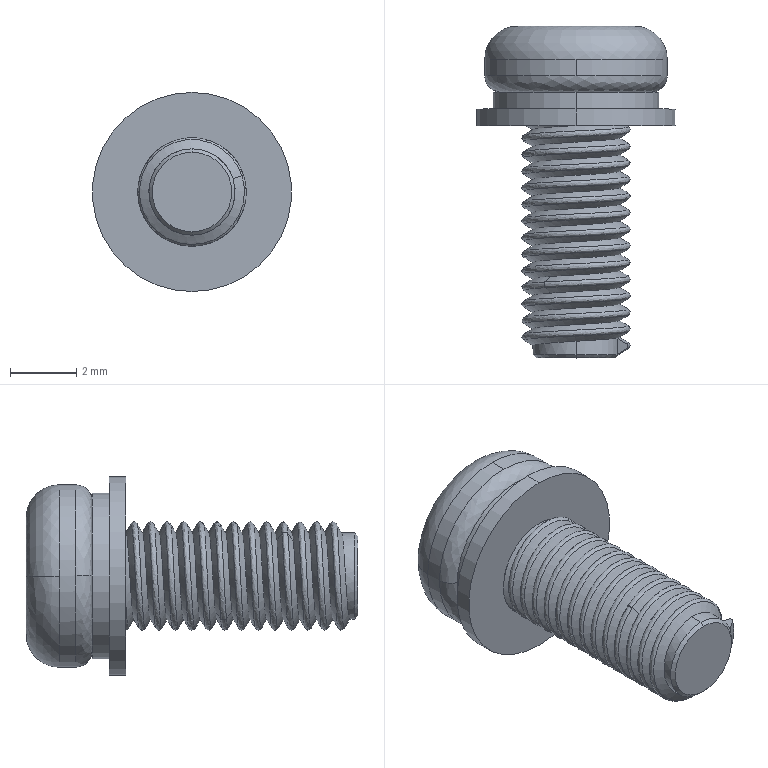Part | SolidWorks | features BaseBody 1 | 1 solid | 58 faces | box 6 x 10 x 6 mm | volume 109.62 mm3 | plane 21 | spline 19 | cylinder 16 | cone 2 | commonest cylinder face diameters 2.6 x5 3 x5 5 x2 5.5 x2 6 x2